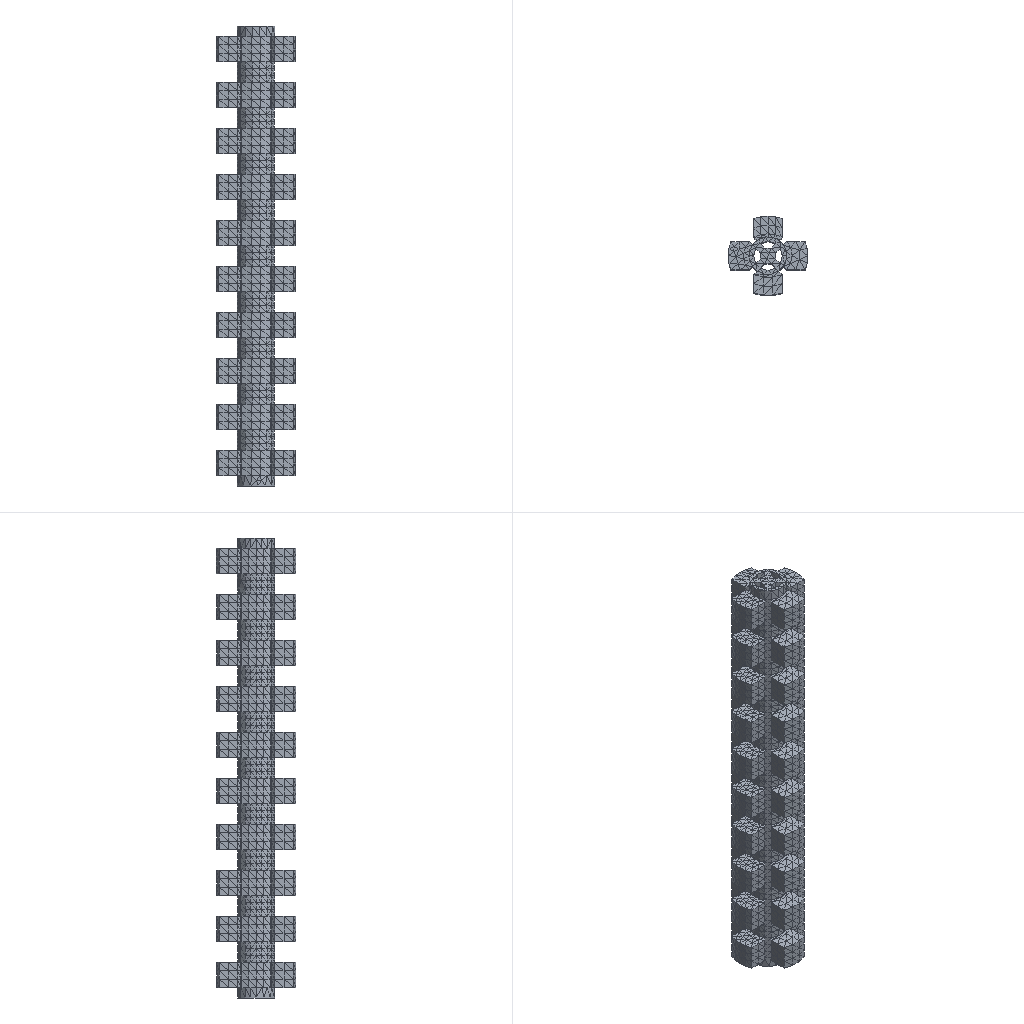Simulation study | abaqus
Set-up summary:
category,name,step,type,value,unit,region
solver,abaqus,,Abaqus/CAE 2024
units,mm-N-s-tonne (MPa),,inferred,E= density=1.07e-09
analysis,Step-1,,dynamic explicit,nlgeom=True; time_period=5
mesh,nodes,,,4923
mesh,elements,,,16129
element_type,C3D4,,,16129
material,Material-1,,density,1.07e-09
material,Material-1,,behaviors,hyperelastic
section,Material-1,,solid section,,,Set-1
load,Load-1,Step-1,pressure,0.0006,,Surf-1
bc,BC-1,Step-1,encastre,[dofs=ENCASTRE],,Set-1
bc,BC-2,Step-1,fixed,"[dofs=ry,rz,x n=3]",,_PickedSet6
contact,Int-1,initial,general contact,interaction=IntProp-1; friction=0.3; behavior=hard
Abaqus input file, long lists of numbers shortened:
*Heading
** Job name: deck Model name: Model-1
** Generated by: Abaqus/CAE 2024
*Preprint, echo=NO, model=NO, history=NO, contact=NO
**
** PARTS
**
*Part, name=qg3
*Node
      1,   3.774,  -8.17,           0.
      2,  -3.774,  -8.17,           0.
** (4921 more lines like these left out)
*Element, type=C3D4
   1, 4786, 2215, 4787, 4788
   2, 4786, 4788, 4789, 2118
** (16127 more lines like these left out)
*Nset, nset=Set-1, generate
    1,  4923,     1
*Elset, elset=Set-1, generate
     1,  16129,      1
** Section: Section-1
*Solid Section, elset=Set-1, material=Material-1
,
*End Part
**
**
** ASSEMBLY
**
*Assembly, name=Assembly
**
*Instance, name=qg3-1, part=qg3
*End Instance
**
*Nset, nset=Set-1, instance=qg3-1
  433,  434,  435,  436,  437,  438,  439,  440,  441,  442,  443,  514,  517,  520,  523,  526
  531,  545,  553,  554,  555,  556, 1842, 1845, 1848, 1850, 1851, 1852, 1853, 2301, 2302, 2303
** (1 more lines like these left out)
*Elset, elset=Set-1, instance=qg3-1
  236,  242,  322,  630,  631,  637,  992,  996, 1396, 1399, 1400, 1406, 1484, 1532, 1542, 1555
 2543, 2548, 2549, 2552, 2553, 2931, 2933, 3376, 3377, 3381, 3383, 3385, 3386, 3389, 3390, 3392
** (1 more lines like these left out)
*Nset, nset=_PickedSet6, internal, instance=qg3-1
  515,  516,  518,  519,  521,  522,  524,  525,  527,  528,  529,  530,  532,  533,  534,  535
  536,  537,  538,  558,  559,  560,  561, 2051, 2166, 2225, 2283, 2284, 2285, 2286, 2287, 2290
** (1 more lines like these left out)
*Elset, elset=_PickedSet6, internal, instance=qg3-1
  283,  387,  392,  540,  543,  687,  696,  764,  768,  971,  998,  999, 1003, 1009, 1011, 1013
 1030, 1559, 1565, 1590, 1591, 1594, 1602, 1607, 1802, 1807, 1808, 1820, 1822, 2072, 2076, 2082
** (1 more lines like these left out)
*Elset, elset=_Surf-1_S2, internal, instance=qg3-1
   195,   280,   792,   793,   825,   851,   858,   863,   878,   889,   902,   911,   917,   932,   959,   981
   985,   987,  1032,  1086,  1087,  1110,  1126,  1201,  1210,  1237,  1265,  1267,  1282,  1304,  1315,  1320
** (7 more lines like these left out)
*Elset, elset=_Surf-1_S1, internal, instance=qg3-1
   124,   125,   272,   338,   640,   643,   734,   791,   812,   831,   834,   849,   875,   890,   910,   927
   931,   945,   952,   955,   980,  1026,  1040,  1044,  1056,  1058,  1130,  1154,  1168,  1173,  1205,  1212
** (9 more lines like these left out)
*Elset, elset=_Surf-1_S4, internal, instance=qg3-1
    72,   486,   512,   524,   824,   882,   891,   946,   966,   968,   986,  1052,  1085,  1128,  1176,  1200
  1209,  1224,  1279,  1286,  1298,  1314,  1329,  1334,  1360,  1408,  1434,  1439,  1456,  1457,  1462,  1471
** (8 more lines like these left out)
*Elset, elset=_Surf-1_S3, internal, instance=qg3-1
    62,   337,   446,   496,   501,   544,   582,   589,   594,   622,   632,   638,   658,   670,   684,   726
   765,   767,   771,   773,   789,   794,   800,   804,   808,   810,   815,   822,   826,   835,   837,   844
** (26 more lines like these left out)
*Surface, type=ELEMENT, name=Surf-1
_Surf-1_S2, S2
_Surf-1_S1, S1
_Surf-1_S4, S4
_Surf-1_S3, S3
*End Assembly
*Amplitude, name=Amp-1
             0.,              0.,              5.,              1.
**
** MATERIALS
**
*Material, name=Material-1
*Density
 1.07e-09,
*Hyperelastic, n=3, ogden
 0.001887,   -3.848,  0.02225,    0.663, 0.003574,    4.225,     2.93,       0.
       0.,
**
** INTERACTION PROPERTIES
**
*Surface Interaction, name=IntProp-1
*Friction
 0.3,
*Surface Behavior, pressure-overclosure=HARD
**
** INTERACTIONS
**
** Interaction: Int-1
*Contact, op=NEW
*Contact Inclusions, ALL EXTERIOR
*Contact Property Assignment
 ,  , IntProp-1
** ----------------------------------------------------------------
**
** STEP: Step-1
**
*Step, name=Step-1, nlgeom=YES
*Dynamic, Explicit
, 5.
*Bulk Viscosity
0.06, 1.2
** Mass Scaling: Semi-Automatic
**               Whole Model
*Variable Mass Scaling, dt=1e-05, type=below min, frequency=1
**
** BOUNDARY CONDITIONS
**
** Name: BC-1 Type: Symmetry/Antisymmetry/Encastre
*Boundary
Set-1, ENCASTRE
** Name: BC-2 Type: Displacement/Rotation
*Boundary
_PickedSet6, 1, 1
_PickedSet6, 5, 5
_PickedSet6, 6, 6
**
** LOADS
**
** Name: Load-1   Type: Pressure
*Dsload, amplitude=Amp-1
Surf-1, P, 0.0006
**
** OUTPUT REQUESTS
**
*Restart, write, number interval=1, time marks=NO
**
** FIELD OUTPUT: F-Output-1
**
*Output, field, variable=PRESELECT, number interval=40
**
** HISTORY OUTPUT: H-Output-1
**
*Output, history, variable=PRESELECT
*End Step
Results summary:
result,odb.job_status,,,JOB_STATUS_UNKNOWN,"consistent, unstated (Abaqus has no unit system)"
result,steps[0].procedure,Step-1,,"*DYNAMIC, EXPLICIT","consistent, unstated (Abaqus has no unit system)"
result,steps[0].time_period,Step-1,,5,"consistent, unstated (Abaqus has no unit system)"
result,steps[0].n_frames,Step-1,,23,"consistent, unstated (Abaqus has no unit system)"
result,steps[0].last_frame.id,Step-1,,274236,"consistent, unstated (Abaqus has no unit system)"
result,steps[0].last_frame.value,Step-1,,2.75,"consistent, unstated (Abaqus has no unit system)"
result,steps[0].last_frame.description,Step-1,,Increment    274236: Step Time =    2.750,"consistent, unstated (Abaqus has no unit system)"
result,steps[0].completed,Step-1,,False,"consistent, unstated (Abaqus has no unit system)"
result,steps[0].max_U_magnitude,Step-1,,337.478,"consistent, unstated (Abaqus has no unit system)"
result,steps[0].max_S_mises,Step-1,,0.04398,"consistent, unstated (Abaqus has no unit system)"
result,steps[0].RF_sum[1],Step-1,,-0.01944,"consistent, unstated (Abaqus has no unit system)"
result,steps[0].RF_sum[2],Step-1,,-0.2643,"consistent, unstated (Abaqus has no unit system)"
result,steps[0].RF_sum[3],Step-1,,-0.133,"consistent, unstated (Abaqus has no unit system)"
result,steps[0].diagnostic.n_increments,Step-1,,25,"consistent, unstated (Abaqus has no unit system)"